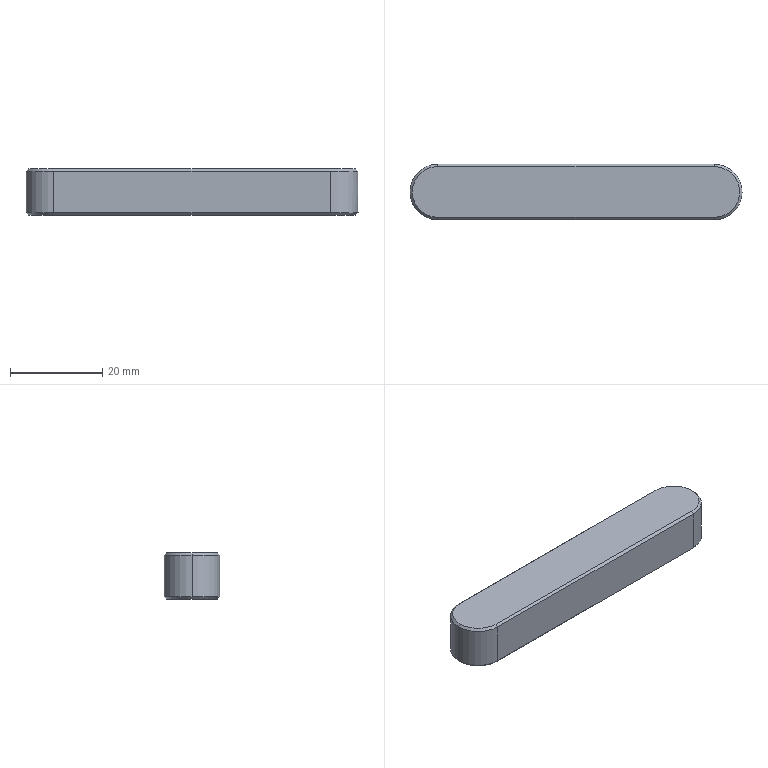Part | SolidWorks | features Chamfer 1, Extrusion 1 | 1 solid | 17 faces | box 72 x 12 x 10 mm | volume 8292 mm3 | plane 8 | cone 6 | cylinder 3 | commonest cylinder face diameters 12 x3
STEP:
#1=CARTESIAN_POINT('',(-5.5,0.,10.));
#2=VERTEX_POINT('',#1);
#3=CARTESIAN_POINT('',(0.,-5.5,10.));
#4=VERTEX_POINT('',#3);
#5=CARTESIAN_POINT('',(0.,0.,10.));
#6=DIRECTION('',(0.,0.,1.));
#7=DIRECTION('',(1.,0.,0.));
#8=AXIS2_PLACEMENT_3D('',#5,#6,#7);
#9=CIRCLE('',#8,5.5);
#10=EDGE_CURVE('',#2,#4,#9,.T.);
#11=ORIENTED_EDGE('',*,*,#10,.F.);
#12=CARTESIAN_POINT('',(-6.,0.,9.5));
#13=VERTEX_POINT('',#12);
#14=CARTESIAN_POINT('',(-5.5,0.,10.));
#15=DIRECTION('',(-0.7071,0.,-0.7071));
#16=VECTOR('',#15,1000.);
#17=LINE('',#14,#16);
#18=EDGE_CURVE('',#2,#13,#17,.T.);
#19=ORIENTED_EDGE('',*,*,#18,.T.);
#20=CARTESIAN_POINT('',(0.,-6.,9.5));
#21=VERTEX_POINT('',#20);
#22=CARTESIAN_POINT('',(0.,0.,9.5));
#23=DIRECTION('',(0.,0.,-1.));
#24=DIRECTION('',(1.,0.,0.));
#25=AXIS2_PLACEMENT_3D('',#22,#23,#24);
#26=CIRCLE('',#25,6.);
#27=EDGE_CURVE('',#21,#13,#26,.T.);
#28=ORIENTED_EDGE('',*,*,#27,.F.);
#29=CARTESIAN_POINT('',(0.,-6.,9.5));
#30=DIRECTION('',(0.,0.7071,0.7071));
#31=VECTOR('',#30,1000.);
#32=LINE('',#29,#31);
#33=EDGE_CURVE('',#21,#4,#32,.T.);
#34=ORIENTED_EDGE('',*,*,#33,.T.);
#35=EDGE_LOOP('',(#11,#19,#28,#34));
#36=FACE_OUTER_BOUND('',#35,.T.);
#37=CARTESIAN_POINT('',(0.,0.,10.));
#38=DIRECTION('',(0.,0.,-1.));
#39=DIRECTION('',(-1.,0.,0.));
#40=AXIS2_PLACEMENT_3D('',#37,#38,#39);
#41=CONICAL_SURFACE('',#40,5.5,0.7854);
#42=ADVANCED_FACE('',(#36),#41,.T.);
#43=CARTESIAN_POINT('',(65.5,0.,0.));
#44=VERTEX_POINT('',#43);
#45=CARTESIAN_POINT('',(60.,-5.5,0.));
#46=VERTEX_POINT('',#45);
#47=CARTESIAN_POINT('',(60.,0.,0.));
#48=DIRECTION('',(0.,0.,-1.));
#49=DIRECTION('',(1.,0.,0.));
#50=AXIS2_PLACEMENT_3D('',#47,#48,#49);
#51=CIRCLE('',#50,5.5);
#52=EDGE_CURVE('',#44,#46,#51,.T.);
#53=ORIENTED_EDGE('',*,*,#52,.F.);
#54=CARTESIAN_POINT('',(66.,0.,0.5));
#55=VERTEX_POINT('',#54);
#56=CARTESIAN_POINT('',(66.,0.,0.5));
#57=DIRECTION('',(0.7071,0.,0.7071));
#58=VECTOR('',#57,1000.);
#59=LINE('',#56,#58);
#60=EDGE_CURVE('',#44,#55,#59,.T.);
#61=ORIENTED_EDGE('',*,*,#60,.T.);
#62=CARTESIAN_POINT('',(60.,-6.,0.5));
#63=VERTEX_POINT('',#62);
#64=CARTESIAN_POINT('',(60.,0.,0.5));
#65=DIRECTION('',(0.,0.,1.));
#66=DIRECTION('',(1.,0.,0.));
#67=AXIS2_PLACEMENT_3D('',#64,#65,#66);
#68=CIRCLE('',#67,6.);
#69=EDGE_CURVE('',#63,#55,#68,.T.);
#70=ORIENTED_EDGE('',*,*,#69,.F.);
#71=CARTESIAN_POINT('',(60.,-5.5,0.));
#72=DIRECTION('',(0.,-0.7071,0.7071));
#73=VECTOR('',#72,1000.);
#74=LINE('',#71,#73);
#75=EDGE_CURVE('',#46,#63,#74,.T.);
#76=ORIENTED_EDGE('',*,*,#75,.F.);
#77=EDGE_LOOP('',(#53,#61,#70,#76));
#78=FACE_OUTER_BOUND('',#77,.T.);
#79=CARTESIAN_POINT('',(60.,0.,0.5));
#80=DIRECTION('',(0.,0.,1.));
#81=DIRECTION('',(1.,0.,0.));
#82=AXIS2_PLACEMENT_3D('',#79,#80,#81);
#83=CONICAL_SURFACE('',#82,6.,0.7854);
#84=ADVANCED_FACE('',(#78),#83,.T.);
#85=ORIENTED_EDGE('',*,*,#27,.T.);
#86=CARTESIAN_POINT('',(-6.,0.,0.5));
#87=VERTEX_POINT('',#86);
#88=CARTESIAN_POINT('',(-6.,0.,10.));
#89=DIRECTION('',(0.,0.,-1.));
#90=VECTOR('',#89,1000.);
#91=LINE('',#88,#90);
#92=EDGE_CURVE('',#13,#87,#91,.T.);
#93=ORIENTED_EDGE('',*,*,#92,.T.);
#94=CARTESIAN_POINT('',(0.,-6.,0.5));
#95=VERTEX_POINT('',#94);
#96=CARTESIAN_POINT('',(0.,0.,0.5));
#97=DIRECTION('',(0.,0.,1.));
#98=DIRECTION('',(1.,0.,0.));
#99=AXIS2_PLACEMENT_3D('',#96,#97,#98);
#100=CIRCLE('',#99,6.);
#101=EDGE_CURVE('',#87,#95,#100,.T.);
#102=ORIENTED_EDGE('',*,*,#101,.T.);
#103=CARTESIAN_POINT('',(0.,-6.,10.));
#104=DIRECTION('',(0.,0.,-1.));
#105=VECTOR('',#104,1000.);
#106=LINE('',#103,#105);
#107=EDGE_CURVE('',#21,#95,#106,.T.);
#108=ORIENTED_EDGE('',*,*,#107,.F.);
#109=EDGE_LOOP('',(#85,#93,#102,#108));
#110=FACE_OUTER_BOUND('',#109,.T.);
#111=CARTESIAN_POINT('',(0.,0.,10.));
#112=DIRECTION('',(0.,0.,-1.));
#113=DIRECTION('',(-1.,0.,0.));
#114=AXIS2_PLACEMENT_3D('',#111,#112,#113);
#115=CYLINDRICAL_SURFACE('',#114,6.);
#116=ADVANCED_FACE('',(#110),#115,.T.);
#117=ORIENTED_EDGE('',*,*,#92,.F.);
#118=CARTESIAN_POINT('',(0.,6.,9.5));
#119=VERTEX_POINT('',#118);
#120=CARTESIAN_POINT('',(0.,0.,9.5));
#121=DIRECTION('',(0.,0.,-1.));
#122=DIRECTION('',(1.,0.,0.));
#123=AXIS2_PLACEMENT_3D('',#120,#121,#122);
#124=CIRCLE('',#123,6.);
#125=EDGE_CURVE('',#13,#119,#124,.T.);
#126=ORIENTED_EDGE('',*,*,#125,.T.);
#127=CARTESIAN_POINT('',(0.,6.,0.5));
#128=VERTEX_POINT('',#127);
#129=CARTESIAN_POINT('',(0.,6.,10.));
#130=DIRECTION('',(0.,0.,-1.));
#131=VECTOR('',#130,1000.);
#132=LINE('',#129,#131);
#133=EDGE_CURVE('',#119,#128,#132,.T.);
#134=ORIENTED_EDGE('',*,*,#133,.T.);
#135=CARTESIAN_POINT('',(0.,0.,0.5));
#136=DIRECTION('',(0.,0.,1.));
#137=DIRECTION('',(1.,0.,0.));
#138=AXIS2_PLACEMENT_3D('',#135,#136,#137);
#139=CIRCLE('',#138,6.);
#140=EDGE_CURVE('',#128,#87,#139,.T.);
#141=ORIENTED_EDGE('',*,*,#140,.T.);
#142=EDGE_LOOP('',(#117,#126,#134,#141));
#143=FACE_OUTER_BOUND('',#142,.T.);
#144=CARTESIAN_POINT('',(0.,0.,10.));
#145=DIRECTION('',(0.,0.,-1.));
#146=DIRECTION('',(-1.,0.,0.));
#147=AXIS2_PLACEMENT_3D('',#144,#145,#146);
#148=CYLINDRICAL_SURFACE('',#147,6.);
#149=ADVANCED_FACE('',(#143),#148,.T.);
#150=ORIENTED_EDGE('',*,*,#107,.T.);
#151=CARTESIAN_POINT('',(0.,-6.,0.5));
#152=DIRECTION('',(1.,0.,0.));
#153=VECTOR('',#152,1000.);
#154=LINE('',#151,#153);
#155=EDGE_CURVE('',#95,#63,#154,.T.);
#156=ORIENTED_EDGE('',*,*,#155,.T.);
#157=CARTESIAN_POINT('',(60.,-6.,9.5));
#158=VERTEX_POINT('',#157);
#159=CARTESIAN_POINT('',(60.,-6.,10.));
#160=DIRECTION('',(0.,0.,-1.));
#161=VECTOR('',#160,1000.);
#162=LINE('',#159,#161);
#163=EDGE_CURVE('',#158,#63,#162,.T.);
#164=ORIENTED_EDGE('',*,*,#163,.F.);
#165=CARTESIAN_POINT('',(0.,-6.,9.5));
#166=DIRECTION('',(-1.,0.,0.));
#167=VECTOR('',#166,1000.);
#168=LINE('',#165,#167);
#169=EDGE_CURVE('',#158,#21,#168,.T.);
#170=ORIENTED_EDGE('',*,*,#169,.T.);
#171=EDGE_LOOP('',(#150,#156,#164,#170));
#172=FACE_OUTER_BOUND('',#171,.T.);
#173=CARTESIAN_POINT('',(0.,-6.,10.));
#174=DIRECTION('',(0.,1.,0.));
#175=DIRECTION('',(0.,0.,1.));
#176=AXIS2_PLACEMENT_3D('',#173,#174,#175);
#177=PLANE('',#176);
#178=ADVANCED_FACE('',(#172),#177,.F.);
#179=ORIENTED_EDGE('',*,*,#163,.T.);
#180=ORIENTED_EDGE('',*,*,#69,.T.);
#181=CARTESIAN_POINT('',(60.,6.,0.5));
#182=VERTEX_POINT('',#181);
#183=CARTESIAN_POINT('',(60.,0.,0.5));
#184=DIRECTION('',(0.,0.,1.));
#185=DIRECTION('',(1.,0.,0.));
#186=AXIS2_PLACEMENT_3D('',#183,#184,#185);
#187=CIRCLE('',#186,6.);
#188=EDGE_CURVE('',#55,#182,#187,.T.);
#189=ORIENTED_EDGE('',*,*,#188,.T.);
#190=CARTESIAN_POINT('',(60.,6.,9.5));
#191=VERTEX_POINT('',#190);
#192=CARTESIAN_POINT('',(60.,6.,10.));
#193=DIRECTION('',(0.,0.,-1.));
#194=VECTOR('',#193,1000.);
#195=LINE('',#192,#194);
#196=EDGE_CURVE('',#191,#182,#195,.T.);
#197=ORIENTED_EDGE('',*,*,#196,.F.);
#198=CARTESIAN_POINT('',(60.,0.,9.5));
#199=DIRECTION('',(0.,0.,-1.));
#200=DIRECTION('',(1.,0.,0.));
#201=AXIS2_PLACEMENT_3D('',#198,#199,#200);
#202=CIRCLE('',#201,6.);
#203=EDGE_CURVE('',#191,#158,#202,.T.);
#204=ORIENTED_EDGE('',*,*,#203,.T.);
#205=EDGE_LOOP('',(#179,#180,#189,#197,#204));
#206=FACE_OUTER_BOUND('',#205,.T.);
#207=CARTESIAN_POINT('',(60.,0.,10.));
#208=DIRECTION('',(0.,0.,-1.));
#209=DIRECTION('',(-1.,0.,0.));
#210=AXIS2_PLACEMENT_3D('',#207,#208,#209);
#211=CYLINDRICAL_SURFACE('',#210,6.);
#212=ADVANCED_FACE('',(#206),#211,.T.);
#213=ORIENTED_EDGE('',*,*,#196,.T.);
#214=CARTESIAN_POINT('',(0.,6.,0.5));
#215=DIRECTION('',(-1.,0.,0.));
#216=VECTOR('',#215,1000.);
#217=LINE('',#214,#216);
#218=EDGE_CURVE('',#182,#128,#217,.T.);
#219=ORIENTED_EDGE('',*,*,#218,.T.);
#220=ORIENTED_EDGE('',*,*,#133,.F.);
#221=CARTESIAN_POINT('',(60.,6.,9.5));
#222=DIRECTION('',(1.,0.,0.));
#223=VECTOR('',#222,1000.);
#224=LINE('',#221,#223);
#225=EDGE_CURVE('',#119,#191,#224,.T.);
#226=ORIENTED_EDGE('',*,*,#225,.T.);
#227=EDGE_LOOP('',(#213,#219,#220,#226));
#228=FACE_OUTER_BOUND('',#227,.T.);
#229=CARTESIAN_POINT('',(0.,6.,10.));
#230=DIRECTION('',(0.,-1.,0.));
#231=DIRECTION('',(0.,0.,-1.));
#232=AXIS2_PLACEMENT_3D('',#229,#230,#231);
#233=PLANE('',#232);
#234=ADVANCED_FACE('',(#228),#233,.F.);
#235=CARTESIAN_POINT('',(60.,-5.5,10.));
#236=VERTEX_POINT('',#235);
#237=CARTESIAN_POINT('',(60.,5.5,10.));
#238=VERTEX_POINT('',#237);
#239=CARTESIAN_POINT('',(60.,0.,10.));
#240=DIRECTION('',(0.,0.,1.));
#241=DIRECTION('',(1.,0.,0.));
#242=AXIS2_PLACEMENT_3D('',#239,#240,#241);
#243=CIRCLE('',#242,5.5);
#244=EDGE_CURVE('',#236,#238,#243,.T.);
#245=ORIENTED_EDGE('',*,*,#244,.T.);
#246=CARTESIAN_POINT('',(0.,5.5,10.));
#247=VERTEX_POINT('',#246);
#248=CARTESIAN_POINT('',(0.,5.5,10.));
#249=DIRECTION('',(-1.,0.,0.));
#250=VECTOR('',#249,1000.);
#251=LINE('',#248,#250);
#252=EDGE_CURVE('',#238,#247,#251,.T.);
#253=ORIENTED_EDGE('',*,*,#252,.T.);
#254=CARTESIAN_POINT('',(0.,0.,10.));
#255=DIRECTION('',(0.,0.,1.));
#256=DIRECTION('',(1.,0.,0.));
#257=AXIS2_PLACEMENT_3D('',#254,#255,#256);
#258=CIRCLE('',#257,5.5);
#259=EDGE_CURVE('',#247,#2,#258,.T.);
#260=ORIENTED_EDGE('',*,*,#259,.T.);
#261=ORIENTED_EDGE('',*,*,#10,.T.);
#262=CARTESIAN_POINT('',(60.,-5.5,10.));
#263=DIRECTION('',(1.,0.,0.));
#264=VECTOR('',#263,1000.);
#265=LINE('',#262,#264);
#266=EDGE_CURVE('',#4,#236,#265,.T.);
#267=ORIENTED_EDGE('',*,*,#266,.T.);
#268=EDGE_LOOP('',(#245,#253,#260,#261,#267));
#269=FACE_OUTER_BOUND('',#268,.T.);
#270=CARTESIAN_POINT('',(0.,0.,10.));
#271=DIRECTION('',(0.,0.,1.));
#272=DIRECTION('',(1.,0.,0.));
#273=AXIS2_PLACEMENT_3D('',#270,#271,#272);
#274=PLANE('',#273);
#275=ADVANCED_FACE('',(#269),#274,.T.);
#276=CARTESIAN_POINT('',(60.,5.5,0.));
#277=VERTEX_POINT('',#276);
#278=CARTESIAN_POINT('',(60.,0.,0.));
#279=DIRECTION('',(0.,0.,-1.));
#280=DIRECTION('',(1.,0.,0.));
#281=AXIS2_PLACEMENT_3D('',#278,#279,#280);
#282=CIRCLE('',#281,5.5);
#283=EDGE_CURVE('',#277,#44,#282,.T.);
#284=ORIENTED_EDGE('',*,*,#283,.T.);
#285=ORIENTED_EDGE('',*,*,#52,.T.);
#286=CARTESIAN_POINT('',(0.,-5.5,0.));
#287=VERTEX_POINT('',#286);
#288=CARTESIAN_POINT('',(0.,-5.5,0.));
#289=DIRECTION('',(-1.,0.,0.));
#290=VECTOR('',#289,1000.);
#291=LINE('',#288,#290);
#292=EDGE_CURVE('',#46,#287,#291,.T.);
#293=ORIENTED_EDGE('',*,*,#292,.T.);
#294=CARTESIAN_POINT('',(0.,5.5,0.));
#295=VERTEX_POINT('',#294);
#296=CARTESIAN_POINT('',(0.,0.,0.));
#297=DIRECTION('',(0.,0.,-1.));
#298=DIRECTION('',(1.,0.,0.));
#299=AXIS2_PLACEMENT_3D('',#296,#297,#298);
#300=CIRCLE('',#299,5.5);
#301=EDGE_CURVE('',#287,#295,#300,.T.);
#302=ORIENTED_EDGE('',*,*,#301,.T.);
#303=CARTESIAN_POINT('',(0.,5.5,0.));
#304=DIRECTION('',(1.,0.,0.));
#305=VECTOR('',#304,1000.);
#306=LINE('',#303,#305);
#307=EDGE_CURVE('',#295,#277,#306,.T.);
#308=ORIENTED_EDGE('',*,*,#307,.T.);
#309=EDGE_LOOP('',(#284,#285,#293,#302,#308));
#310=FACE_OUTER_BOUND('',#309,.T.);
#311=CARTESIAN_POINT('',(0.,0.,0.));
#312=DIRECTION('',(0.,0.,1.));
#313=DIRECTION('',(1.,0.,0.));
#314=AXIS2_PLACEMENT_3D('',#311,#312,#313);
#315=PLANE('',#314);
#316=ADVANCED_FACE('',(#310),#315,.F.);
#317=CARTESIAN_POINT('',(60.,5.5,0.));
#318=DIRECTION('',(0.,0.7071,0.7071));
#319=VECTOR('',#318,1000.);
#320=LINE('',#317,#319);
#321=EDGE_CURVE('',#277,#182,#320,.T.);
#322=ORIENTED_EDGE('',*,*,#321,.F.);
#323=ORIENTED_EDGE('',*,*,#307,.F.);
#324=CARTESIAN_POINT('',(0.,6.,0.5));
#325=DIRECTION('',(0.,-0.7071,-0.7071));
#326=VECTOR('',#325,1000.);
#327=LINE('',#324,#326);
#328=EDGE_CURVE('',#128,#295,#327,.T.);
#329=ORIENTED_EDGE('',*,*,#328,.F.);
#330=ORIENTED_EDGE('',*,*,#218,.F.);
#331=EDGE_LOOP('',(#322,#323,#329,#330));
#332=FACE_OUTER_BOUND('',#331,.T.);
#333=CARTESIAN_POINT('',(0.,6.,0.5));
#334=DIRECTION('',(0.,-0.7071,0.7071));
#335=DIRECTION('',(-1.,0.,0.));
#336=AXIS2_PLACEMENT_3D('',#333,#334,#335);
#337=PLANE('',#336);
#338=ADVANCED_FACE('',(#332),#337,.F.);
#339=ORIENTED_EDGE('',*,*,#328,.T.);
#340=ORIENTED_EDGE('',*,*,#301,.F.);
#341=CARTESIAN_POINT('',(0.,-6.,0.5));
#342=DIRECTION('',(0.,0.7071,-0.7071));
#343=VECTOR('',#342,1000.);
#344=LINE('',#341,#343);
#345=EDGE_CURVE('',#95,#287,#344,.T.);
#346=ORIENTED_EDGE('',*,*,#345,.F.);
#347=ORIENTED_EDGE('',*,*,#101,.F.);
#348=ORIENTED_EDGE('',*,*,#140,.F.);
#349=EDGE_LOOP('',(#339,#340,#346,#347,#348));
#350=FACE_OUTER_BOUND('',#349,.T.);
#351=CARTESIAN_POINT('',(0.,0.,0.5));
#352=DIRECTION('',(0.,0.,1.));
#353=DIRECTION('',(1.,0.,0.));
#354=AXIS2_PLACEMENT_3D('',#351,#352,#353);
#355=CONICAL_SURFACE('',#354,6.,0.7854);
#356=ADVANCED_FACE('',(#350),#355,.T.);
#357=ORIENTED_EDGE('',*,*,#60,.F.);
#358=ORIENTED_EDGE('',*,*,#283,.F.);
#359=ORIENTED_EDGE('',*,*,#321,.T.);
#360=ORIENTED_EDGE('',*,*,#188,.F.);
#361=EDGE_LOOP('',(#357,#358,#359,#360));
#362=FACE_OUTER_BOUND('',#361,.T.);
#363=CARTESIAN_POINT('',(60.,0.,0.5));
#364=DIRECTION('',(0.,0.,1.));
#365=DIRECTION('',(1.,0.,0.));
#366=AXIS2_PLACEMENT_3D('',#363,#364,#365);
#367=CONICAL_SURFACE('',#366,6.,0.7854);
#368=ADVANCED_FACE('',(#362),#367,.T.);
#369=ORIENTED_EDGE('',*,*,#345,.T.);
#370=ORIENTED_EDGE('',*,*,#292,.F.);
#371=ORIENTED_EDGE('',*,*,#75,.T.);
#372=ORIENTED_EDGE('',*,*,#155,.F.);
#373=EDGE_LOOP('',(#369,#370,#371,#372));
#374=FACE_OUTER_BOUND('',#373,.T.);
#375=CARTESIAN_POINT('',(0.,-6.,0.5));
#376=DIRECTION('',(0.,0.7071,0.7071));
#377=DIRECTION('',(1.,0.,0.));
#378=AXIS2_PLACEMENT_3D('',#375,#376,#377);
#379=PLANE('',#378);
#380=ADVANCED_FACE('',(#374),#379,.F.);
#381=ORIENTED_EDGE('',*,*,#33,.F.);
#382=ORIENTED_EDGE('',*,*,#169,.F.);
#383=CARTESIAN_POINT('',(60.,-5.5,10.));
#384=DIRECTION('',(0.,-0.7071,-0.7071));
#385=VECTOR('',#384,1000.);
#386=LINE('',#383,#385);
#387=EDGE_CURVE('',#236,#158,#386,.T.);
#388=ORIENTED_EDGE('',*,*,#387,.F.);
#389=ORIENTED_EDGE('',*,*,#266,.F.);
#390=EDGE_LOOP('',(#381,#382,#388,#389));
#391=FACE_OUTER_BOUND('',#390,.T.);
#392=CARTESIAN_POINT('',(0.,-5.5,10.));
#393=DIRECTION('',(0.,-0.7071,0.7071));
#394=DIRECTION('',(-1.,0.,0.));
#395=AXIS2_PLACEMENT_3D('',#392,#393,#394);
#396=PLANE('',#395);
#397=ADVANCED_FACE('',(#391),#396,.T.);
#398=ORIENTED_EDGE('',*,*,#387,.T.);
#399=ORIENTED_EDGE('',*,*,#203,.F.);
#400=CARTESIAN_POINT('',(60.,5.5,10.));
#401=DIRECTION('',(0.,0.7071,-0.7071));
#402=VECTOR('',#401,1000.);
#403=LINE('',#400,#402);
#404=EDGE_CURVE('',#238,#191,#403,.T.);
#405=ORIENTED_EDGE('',*,*,#404,.F.);
#406=ORIENTED_EDGE('',*,*,#244,.F.);
#407=EDGE_LOOP('',(#398,#399,#405,#406));
#408=FACE_OUTER_BOUND('',#407,.T.);
#409=CARTESIAN_POINT('',(60.,0.,10.));
#410=DIRECTION('',(0.,0.,-1.));
#411=DIRECTION('',(-1.,0.,0.));
#412=AXIS2_PLACEMENT_3D('',#409,#410,#411);
#413=CONICAL_SURFACE('',#412,5.5,0.7854);
#414=ADVANCED_FACE('',(#408),#413,.T.);
#415=ORIENTED_EDGE('',*,*,#18,.F.);
#416=ORIENTED_EDGE('',*,*,#259,.F.);
#417=CARTESIAN_POINT('',(0.,6.,9.5));
#418=DIRECTION('',(0.,-0.7071,0.7071));
#419=VECTOR('',#418,1000.);
#420=LINE('',#417,#419);
#421=EDGE_CURVE('',#119,#247,#420,.T.);
#422=ORIENTED_EDGE('',*,*,#421,.F.);
#423=ORIENTED_EDGE('',*,*,#125,.F.);
#424=EDGE_LOOP('',(#415,#416,#422,#423));
#425=FACE_OUTER_BOUND('',#424,.T.);
#426=CARTESIAN_POINT('',(0.,0.,10.));
#427=DIRECTION('',(0.,0.,-1.));
#428=DIRECTION('',(-1.,0.,0.));
#429=AXIS2_PLACEMENT_3D('',#426,#427,#428);
#430=CONICAL_SURFACE('',#429,5.5,0.7854);
#431=ADVANCED_FACE('',(#425),#430,.T.);
#432=ORIENTED_EDGE('',*,*,#404,.T.);
#433=ORIENTED_EDGE('',*,*,#225,.F.);
#434=ORIENTED_EDGE('',*,*,#421,.T.);
#435=ORIENTED_EDGE('',*,*,#252,.F.);
#436=EDGE_LOOP('',(#432,#433,#434,#435));
#437=FACE_OUTER_BOUND('',#436,.T.);
#438=CARTESIAN_POINT('',(0.,5.5,10.));
#439=DIRECTION('',(0.,0.7071,0.7071));
#440=DIRECTION('',(1.,0.,0.));
#441=AXIS2_PLACEMENT_3D('',#438,#439,#440);
#442=PLANE('',#441);
#443=ADVANCED_FACE('',(#437),#442,.T.);
#444=CLOSED_SHELL('',(#42,#84,#116,#149,#178,#212,#234,#275,#316,#338,#356,#368,#380,#397,#414,#431,#443));
#445=MANIFOLD_SOLID_BREP('',#444);
#446=CARTESIAN_POINT('',(0.,0.,0.));
#447=DIRECTION('',(0.,0.,1.));
#448=DIRECTION('',(1.,0.,0.));
#449=AXIS2_PLACEMENT_3D('',#446,#447,#448);
#450=(LENGTH_UNIT()NAMED_UNIT(*)SI_UNIT(.MILLI.,.METRE.));
#451=UNCERTAINTY_MEASURE_WITH_UNIT(LENGTH_MEASURE(0.00001),#450,'','');
#452=(NAMED_UNIT(*)PLANE_ANGLE_UNIT()SI_UNIT($,.RADIAN.));
#453=(NAMED_UNIT(*)SI_UNIT($,.STERADIAN.)SOLID_ANGLE_UNIT());
#454=(GEOMETRIC_REPRESENTATION_CONTEXT(3)GLOBAL_UNCERTAINTY_ASSIGNED_CONTEXT((#451))GLOBAL_UNIT_ASSIGNED_CONTEXT((#450,#452,#453))REPRESENTATION_CONTEXT('',''));
#455=ADVANCED_BREP_SHAPE_REPRESENTATION('',(#445,#449),#454);